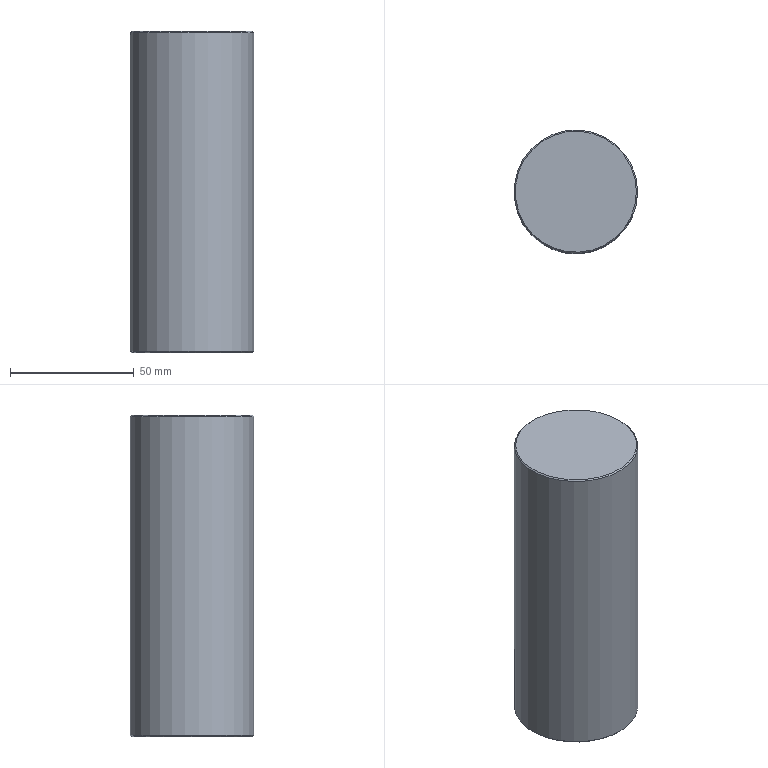Part | STEP file | solid 177 | 1 solid | 7 faces | box 50 x 50 x 130 mm | volume 253962 mm3 | cone 3 | plane 2 | cylinder 2 | commonest cylinder face diameters 10 x1 50 x1